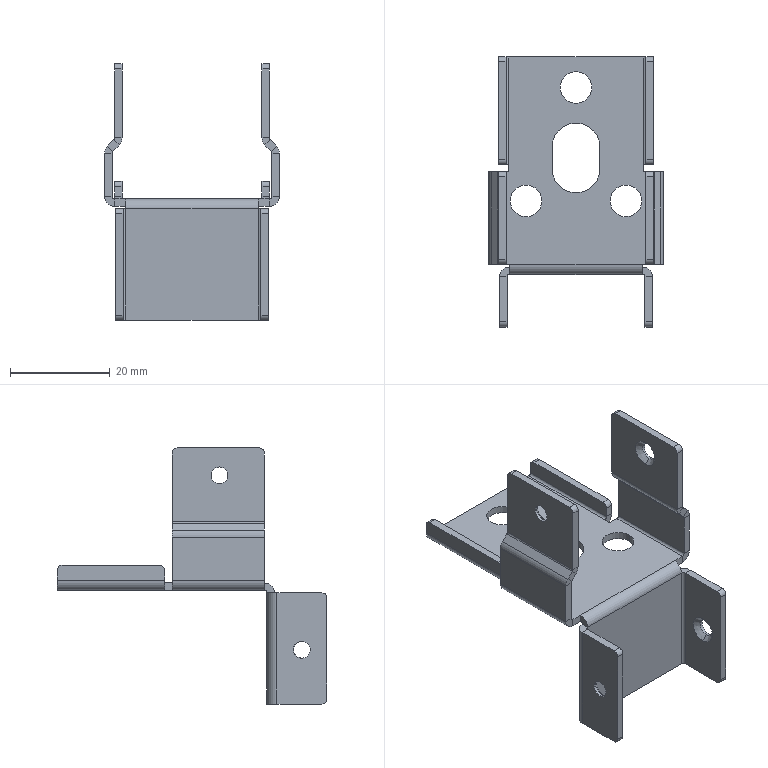Part | NX | features solid 2 | 1 solid | 136 faces | box 35 x 54 x 51.24 mm | volume 5099 mm3 | plane 78 | cylinder 50 | cone 8 | commonest cylinder face diameters 2 x12 1 x11 4 x11 3.4 x8 6.35 x6 9.5 x2